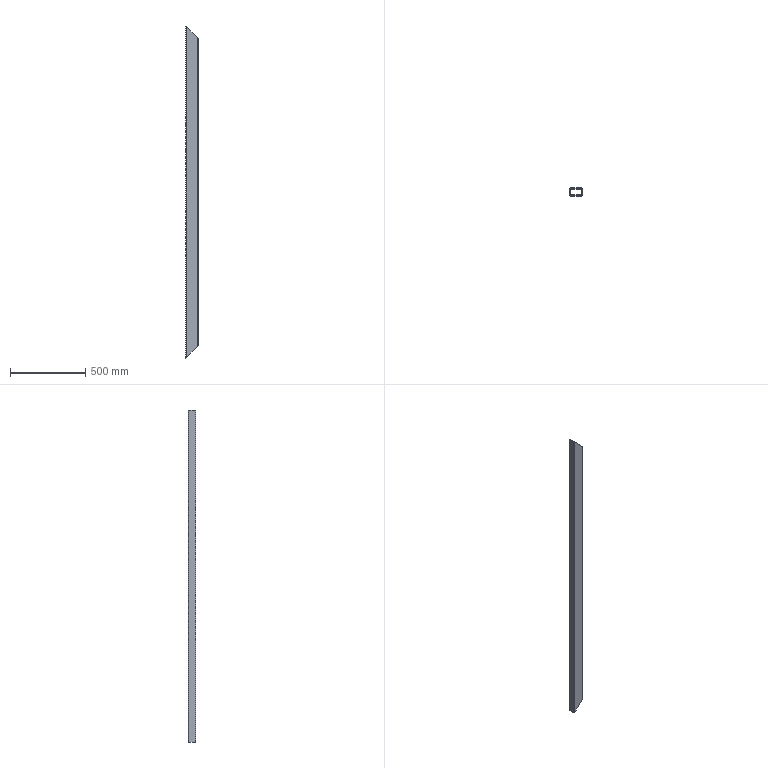Part | SolidWorks | features Extrusion 1, ICE 1, Shell 1 | 1 solid | 18 faces | box 80 x 50 x 2200 mm | volume 2025444 mm3 | plane 10 | cylinder 8 | commonest cylinder face diameters 2 x4 10 x4
STEP:
#1=CARTESIAN_POINT('',(-35.,21.,2195.));
#2=VERTEX_POINT('',#1);
#3=CARTESIAN_POINT('',(35.,21.,2125.));
#4=VERTEX_POINT('',#3);
#5=CARTESIAN_POINT('',(-2.5,21.,2162.5));
#6=DIRECTION('',(0.7071,0.,-0.7071));
#7=VECTOR('',#6,1000.);
#8=LINE('',#5,#7);
#9=EDGE_CURVE('',#2,#4,#8,.T.);
#10=ORIENTED_EDGE('',*,*,#9,.F.);
#11=CARTESIAN_POINT('',(-35.,21.,5.));
#12=VERTEX_POINT('',#11);
#13=CARTESIAN_POINT('',(-35.,21.,2200.));
#14=DIRECTION('',(0.,0.,-1.));
#15=VECTOR('',#14,1000.);
#16=LINE('',#13,#15);
#17=EDGE_CURVE('',#2,#12,#16,.T.);
#18=ORIENTED_EDGE('',*,*,#17,.T.);
#19=CARTESIAN_POINT('',(35.,21.,75.));
#20=VERTEX_POINT('',#19);
#21=CARTESIAN_POINT('',(1097.5,21.,1137.5));
#22=DIRECTION('',(-0.7071,0.,-0.7071));
#23=VECTOR('',#22,1000.);
#24=LINE('',#21,#23);
#25=EDGE_CURVE('',#20,#12,#24,.T.);
#26=ORIENTED_EDGE('',*,*,#25,.F.);
#27=CARTESIAN_POINT('',(35.,21.,2200.));
#28=DIRECTION('',(0.,0.,-1.));
#29=VECTOR('',#28,1000.);
#30=LINE('',#27,#29);
#31=EDGE_CURVE('',#4,#20,#30,.T.);
#32=ORIENTED_EDGE('',*,*,#31,.F.);
#33=EDGE_LOOP('',(#10,#18,#26,#32));
#34=FACE_OUTER_BOUND('',#33,.T.);
#35=CARTESIAN_POINT('',(35.,21.,2200.));
#36=DIRECTION('',(0.,-1.,0.));
#37=DIRECTION('',(1.,0.,0.));
#38=AXIS2_PLACEMENT_3D('',#35,#36,#37);
#39=PLANE('',#38);
#40=ADVANCED_FACE('',(#34),#39,.T.);
#41=CARTESIAN_POINT('',(36.,20.,2124.));
#42=VERTEX_POINT('',#41);
#43=CARTESIAN_POINT('',(36.,20.,76.));
#44=VERTEX_POINT('',#43);
#45=CARTESIAN_POINT('',(36.,20.,2200.));
#46=DIRECTION('',(0.,0.,-1.));
#47=VECTOR('',#46,1000.);
#48=LINE('',#45,#47);
#49=EDGE_CURVE('',#42,#44,#48,.T.);
#50=ORIENTED_EDGE('',*,*,#49,.F.);
#51=CARTESIAN_POINT('',(36.,20.,2124.));
#52=CARTESIAN_POINT('',(36.,20.586,2124.));
#53=CARTESIAN_POINT('',(35.586,21.,2124.414));
#54=CARTESIAN_POINT('',(35.,21.,2125.));
#55=(BOUNDED_CURVE()B_SPLINE_CURVE(3,(#51,#52,#53,#54),.UNSPECIFIED.,.F.,.T.)B_SPLINE_CURVE_WITH_KNOTS((4,4),(0.,1.571),.UNSPECIFIED.)CURVE()GEOMETRIC_REPRESENTATION_ITEM()RATIONAL_B_SPLINE_CURVE((1.,0.8047,0.8047,1.))REPRESENTATION_ITEM(''));
#56=EDGE_CURVE('',#42,#4,#55,.T.);
#57=ORIENTED_EDGE('',*,*,#56,.T.);
#58=ORIENTED_EDGE('',*,*,#31,.T.);
#59=CARTESIAN_POINT('',(35.,21.,75.));
#60=CARTESIAN_POINT('',(35.586,21.,75.586));
#61=CARTESIAN_POINT('',(36.,20.586,76.));
#62=CARTESIAN_POINT('',(36.,20.,76.));
#63=(BOUNDED_CURVE()B_SPLINE_CURVE(3,(#59,#60,#61,#62),.UNSPECIFIED.,.F.,.F.)B_SPLINE_CURVE_WITH_KNOTS((4,4),(1.571,3.142),.UNSPECIFIED.)CURVE()GEOMETRIC_REPRESENTATION_ITEM()RATIONAL_B_SPLINE_CURVE((1.,0.8047,0.8047,1.))REPRESENTATION_ITEM(''));
#64=EDGE_CURVE('',#20,#44,#63,.T.);
#65=ORIENTED_EDGE('',*,*,#64,.T.);
#66=EDGE_LOOP('',(#50,#57,#58,#65));
#67=FACE_OUTER_BOUND('',#66,.T.);
#68=CARTESIAN_POINT('',(35.,20.,2200.));
#69=DIRECTION('',(0.,0.,-1.));
#70=DIRECTION('',(-1.,0.,0.));
#71=AXIS2_PLACEMENT_3D('',#68,#69,#70);
#72=CYLINDRICAL_SURFACE('',#71,1.);
#73=ADVANCED_FACE('',(#67),#72,.F.);
#74=CARTESIAN_POINT('',(36.,-20.,2124.));
#75=VERTEX_POINT('',#74);
#76=CARTESIAN_POINT('',(36.,-20.,76.));
#77=VERTEX_POINT('',#76);
#78=CARTESIAN_POINT('',(36.,-20.,2200.));
#79=DIRECTION('',(0.,0.,-1.));
#80=VECTOR('',#79,1000.);
#81=LINE('',#78,#80);
#82=EDGE_CURVE('',#75,#77,#81,.T.);
#83=ORIENTED_EDGE('',*,*,#82,.F.);
#84=CARTESIAN_POINT('',(36.,20.,2124.));
#85=DIRECTION('',(0.,1.,0.));
#86=VECTOR('',#85,1000.);
#87=LINE('',#84,#86);
#88=EDGE_CURVE('',#75,#42,#87,.T.);
#89=ORIENTED_EDGE('',*,*,#88,.T.);
#90=ORIENTED_EDGE('',*,*,#49,.T.);
#91=CARTESIAN_POINT('',(36.,20.,76.));
#92=DIRECTION('',(0.,-1.,0.));
#93=VECTOR('',#92,1000.);
#94=LINE('',#91,#93);
#95=EDGE_CURVE('',#44,#77,#94,.T.);
#96=ORIENTED_EDGE('',*,*,#95,.T.);
#97=EDGE_LOOP('',(#83,#89,#90,#96));
#98=FACE_OUTER_BOUND('',#97,.T.);
#99=CARTESIAN_POINT('',(36.,20.,2200.));
#100=DIRECTION('',(1.,0.,0.));
#101=DIRECTION('',(0.,1.,0.));
#102=AXIS2_PLACEMENT_3D('',#99,#100,#101);
#103=PLANE('',#102);
#104=ADVANCED_FACE('',(#98),#103,.F.);
#105=CARTESIAN_POINT('',(35.,-21.,2125.));
#106=VERTEX_POINT('',#105);
#107=CARTESIAN_POINT('',(35.,-21.,75.));
#108=VERTEX_POINT('',#107);
#109=CARTESIAN_POINT('',(35.,-21.,2200.));
#110=DIRECTION('',(0.,0.,-1.));
#111=VECTOR('',#110,1000.);
#112=LINE('',#109,#111);
#113=EDGE_CURVE('',#106,#108,#112,.T.);
#114=ORIENTED_EDGE('',*,*,#113,.F.);
#115=CARTESIAN_POINT('',(35.,-21.,2125.));
#116=CARTESIAN_POINT('',(35.586,-21.,2124.414));
#117=CARTESIAN_POINT('',(36.,-20.586,2124.));
#118=CARTESIAN_POINT('',(36.,-20.,2124.));
#119=(BOUNDED_CURVE()B_SPLINE_CURVE(3,(#115,#116,#117,#118),.UNSPECIFIED.,.F.,.T.)B_SPLINE_CURVE_WITH_KNOTS((4,4),(4.712,6.283),.UNSPECIFIED.)CURVE()GEOMETRIC_REPRESENTATION_ITEM()RATIONAL_B_SPLINE_CURVE((1.,0.8047,0.8047,1.))REPRESENTATION_ITEM(''));
#120=EDGE_CURVE('',#106,#75,#119,.T.);
#121=ORIENTED_EDGE('',*,*,#120,.T.);
#122=ORIENTED_EDGE('',*,*,#82,.T.);
#123=CARTESIAN_POINT('',(36.,-20.,76.));
#124=CARTESIAN_POINT('',(36.,-20.586,76.));
#125=CARTESIAN_POINT('',(35.586,-21.,75.586));
#126=CARTESIAN_POINT('',(35.,-21.,75.));
#127=(BOUNDED_CURVE()B_SPLINE_CURVE(3,(#123,#124,#125,#126),.UNSPECIFIED.,.F.,.T.)B_SPLINE_CURVE_WITH_KNOTS((4,4),(3.142,4.712),.UNSPECIFIED.)CURVE()GEOMETRIC_REPRESENTATION_ITEM()RATIONAL_B_SPLINE_CURVE((1.,0.8047,0.8047,1.))REPRESENTATION_ITEM(''));
#128=EDGE_CURVE('',#77,#108,#127,.T.);
#129=ORIENTED_EDGE('',*,*,#128,.T.);
#130=EDGE_LOOP('',(#114,#121,#122,#129));
#131=FACE_OUTER_BOUND('',#130,.T.);
#132=CARTESIAN_POINT('',(35.,-20.,2200.));
#133=DIRECTION('',(0.,0.,-1.));
#134=DIRECTION('',(-1.,0.,0.));
#135=AXIS2_PLACEMENT_3D('',#132,#133,#134);
#136=CYLINDRICAL_SURFACE('',#135,1.);
#137=ADVANCED_FACE('',(#131),#136,.F.);
#138=CARTESIAN_POINT('',(-35.,-21.,2195.));
#139=VERTEX_POINT('',#138);
#140=CARTESIAN_POINT('',(-35.,-21.,5.));
#141=VERTEX_POINT('',#140);
#142=CARTESIAN_POINT('',(-35.,-21.,2200.));
#143=DIRECTION('',(0.,0.,-1.));
#144=VECTOR('',#143,1000.);
#145=LINE('',#142,#144);
#146=EDGE_CURVE('',#139,#141,#145,.T.);
#147=ORIENTED_EDGE('',*,*,#146,.F.);
#148=CARTESIAN_POINT('',(-2.5,-21.,2162.5));
#149=DIRECTION('',(0.7071,0.,-0.7071));
#150=VECTOR('',#149,1000.);
#151=LINE('',#148,#150);
#152=EDGE_CURVE('',#139,#106,#151,.T.);
#153=ORIENTED_EDGE('',*,*,#152,.T.);
#154=ORIENTED_EDGE('',*,*,#113,.T.);
#155=CARTESIAN_POINT('',(1097.5,-21.,1137.5));
#156=DIRECTION('',(-0.7071,0.,-0.7071));
#157=VECTOR('',#156,1000.);
#158=LINE('',#155,#157);
#159=EDGE_CURVE('',#108,#141,#158,.T.);
#160=ORIENTED_EDGE('',*,*,#159,.T.);
#161=EDGE_LOOP('',(#147,#153,#154,#160));
#162=FACE_OUTER_BOUND('',#161,.T.);
#163=CARTESIAN_POINT('',(35.,-21.,2200.));
#164=DIRECTION('',(0.,-1.,0.));
#165=DIRECTION('',(1.,0.,0.));
#166=AXIS2_PLACEMENT_3D('',#163,#164,#165);
#167=PLANE('',#166);
#168=ADVANCED_FACE('',(#162),#167,.F.);
#169=CARTESIAN_POINT('',(-36.,-20.,2196.));
#170=VERTEX_POINT('',#169);
#171=CARTESIAN_POINT('',(-36.,-20.,4.));
#172=VERTEX_POINT('',#171);
#173=CARTESIAN_POINT('',(-36.,-20.,2200.));
#174=DIRECTION('',(0.,0.,-1.));
#175=VECTOR('',#174,1000.);
#176=LINE('',#173,#175);
#177=EDGE_CURVE('',#170,#172,#176,.T.);
#178=ORIENTED_EDGE('',*,*,#177,.F.);
#179=CARTESIAN_POINT('',(-36.,-20.,2196.));
#180=CARTESIAN_POINT('',(-36.,-20.586,2196.));
#181=CARTESIAN_POINT('',(-35.586,-21.,2195.586));
#182=CARTESIAN_POINT('',(-35.,-21.,2195.));
#183=(BOUNDED_CURVE()B_SPLINE_CURVE(3,(#179,#180,#181,#182),.UNSPECIFIED.,.F.,.T.)B_SPLINE_CURVE_WITH_KNOTS((4,4),(3.142,4.712),.UNSPECIFIED.)CURVE()GEOMETRIC_REPRESENTATION_ITEM()RATIONAL_B_SPLINE_CURVE((1.,0.8047,0.8047,1.))REPRESENTATION_ITEM(''));
#184=EDGE_CURVE('',#170,#139,#183,.T.);
#185=ORIENTED_EDGE('',*,*,#184,.T.);
#186=ORIENTED_EDGE('',*,*,#146,.T.);
#187=CARTESIAN_POINT('',(-35.,-21.,5.));
#188=CARTESIAN_POINT('',(-35.586,-21.,4.414));
#189=CARTESIAN_POINT('',(-36.,-20.586,4.));
#190=CARTESIAN_POINT('',(-36.,-20.,4.));
#191=(BOUNDED_CURVE()B_SPLINE_CURVE(3,(#187,#188,#189,#190),.UNSPECIFIED.,.F.,.T.)B_SPLINE_CURVE_WITH_KNOTS((4,4),(4.712,6.283),.UNSPECIFIED.)CURVE()GEOMETRIC_REPRESENTATION_ITEM()RATIONAL_B_SPLINE_CURVE((1.,0.8047,0.8047,1.))REPRESENTATION_ITEM(''));
#192=EDGE_CURVE('',#141,#172,#191,.T.);
#193=ORIENTED_EDGE('',*,*,#192,.T.);
#194=EDGE_LOOP('',(#178,#185,#186,#193));
#195=FACE_OUTER_BOUND('',#194,.T.);
#196=CARTESIAN_POINT('',(-35.,-20.,2200.));
#197=DIRECTION('',(0.,0.,-1.));
#198=DIRECTION('',(-1.,0.,0.));
#199=AXIS2_PLACEMENT_3D('',#196,#197,#198);
#200=CYLINDRICAL_SURFACE('',#199,1.);
#201=ADVANCED_FACE('',(#195),#200,.F.);
#202=CARTESIAN_POINT('',(-36.,20.,2196.));
#203=VERTEX_POINT('',#202);
#204=CARTESIAN_POINT('',(-36.,20.,2196.));
#205=DIRECTION('',(0.,1.,0.));
#206=VECTOR('',#205,1000.);
#207=LINE('',#204,#206);
#208=EDGE_CURVE('',#170,#203,#207,.T.);
#209=ORIENTED_EDGE('',*,*,#208,.F.);
#210=ORIENTED_EDGE('',*,*,#177,.T.);
#211=CARTESIAN_POINT('',(-36.,20.,4.));
#212=VERTEX_POINT('',#211);
#213=CARTESIAN_POINT('',(-36.,20.,4.));
#214=DIRECTION('',(0.,-1.,0.));
#215=VECTOR('',#214,1000.);
#216=LINE('',#213,#215);
#217=EDGE_CURVE('',#212,#172,#216,.T.);
#218=ORIENTED_EDGE('',*,*,#217,.F.);
#219=CARTESIAN_POINT('',(-36.,20.,2200.));
#220=DIRECTION('',(0.,0.,-1.));
#221=VECTOR('',#220,1000.);
#222=LINE('',#219,#221);
#223=EDGE_CURVE('',#203,#212,#222,.T.);
#224=ORIENTED_EDGE('',*,*,#223,.F.);
#225=EDGE_LOOP('',(#209,#210,#218,#224));
#226=FACE_OUTER_BOUND('',#225,.T.);
#227=CARTESIAN_POINT('',(-36.,20.,2200.));
#228=DIRECTION('',(1.,0.,0.));
#229=DIRECTION('',(0.,1.,0.));
#230=AXIS2_PLACEMENT_3D('',#227,#228,#229);
#231=PLANE('',#230);
#232=ADVANCED_FACE('',(#226),#231,.T.);
#233=CARTESIAN_POINT('',(-36.,20.,2196.));
#234=CARTESIAN_POINT('',(-36.,20.586,2196.));
#235=CARTESIAN_POINT('',(-35.586,21.,2195.586));
#236=CARTESIAN_POINT('',(-35.,21.,2195.));
#237=(BOUNDED_CURVE()B_SPLINE_CURVE(3,(#233,#234,#235,#236),.UNSPECIFIED.,.F.,.T.)B_SPLINE_CURVE_WITH_KNOTS((4,4),(3.142,4.712),.UNSPECIFIED.)CURVE()GEOMETRIC_REPRESENTATION_ITEM()RATIONAL_B_SPLINE_CURVE((1.,0.8047,0.8047,1.))REPRESENTATION_ITEM(''));
#238=EDGE_CURVE('',#203,#2,#237,.T.);
#239=ORIENTED_EDGE('',*,*,#238,.F.);
#240=ORIENTED_EDGE('',*,*,#223,.T.);
#241=CARTESIAN_POINT('',(-35.,21.,5.));
#242=CARTESIAN_POINT('',(-35.586,21.,4.414));
#243=CARTESIAN_POINT('',(-36.,20.586,4.));
#244=CARTESIAN_POINT('',(-36.,20.,4.));
#245=(BOUNDED_CURVE()B_SPLINE_CURVE(3,(#241,#242,#243,#244),.UNSPECIFIED.,.F.,.T.)B_SPLINE_CURVE_WITH_KNOTS((4,4),(4.712,6.283),.UNSPECIFIED.)CURVE()GEOMETRIC_REPRESENTATION_ITEM()RATIONAL_B_SPLINE_CURVE((1.,0.8047,0.8047,1.))REPRESENTATION_ITEM(''));
#246=EDGE_CURVE('',#12,#212,#245,.T.);
#247=ORIENTED_EDGE('',*,*,#246,.F.);
#248=ORIENTED_EDGE('',*,*,#17,.F.);
#249=EDGE_LOOP('',(#239,#240,#247,#248));
#250=FACE_OUTER_BOUND('',#249,.T.);
#251=CARTESIAN_POINT('',(-35.,20.,2200.));
#252=DIRECTION('',(0.,0.,-1.));
#253=DIRECTION('',(-1.,0.,0.));
#254=AXIS2_PLACEMENT_3D('',#251,#252,#253);
#255=CYLINDRICAL_SURFACE('',#254,1.);
#256=ADVANCED_FACE('',(#250),#255,.F.);
#257=CARTESIAN_POINT('',(-35.,-25.,5.));
#258=VERTEX_POINT('',#257);
#259=CARTESIAN_POINT('',(-40.,-20.,0.));
#260=VERTEX_POINT('',#259);
#261=CARTESIAN_POINT('',(-35.,-25.,5.));
#262=CARTESIAN_POINT('',(-37.929,-25.,2.071));
#263=CARTESIAN_POINT('',(-40.,-22.929,0.));
#264=CARTESIAN_POINT('',(-40.,-20.,0.));
#265=(BOUNDED_CURVE()B_SPLINE_CURVE(3,(#261,#262,#263,#264),.UNSPECIFIED.,.F.,.T.)B_SPLINE_CURVE_WITH_KNOTS((4,4),(4.712,6.283),.UNSPECIFIED.)CURVE()GEOMETRIC_REPRESENTATION_ITEM()RATIONAL_B_SPLINE_CURVE((1.,0.8047,0.8047,1.))REPRESENTATION_ITEM(''));
#266=EDGE_CURVE('',#258,#260,#265,.T.);
#267=ORIENTED_EDGE('',*,*,#266,.T.);
#268=CARTESIAN_POINT('',(-40.,20.,0.));
#269=VERTEX_POINT('',#268);
#270=CARTESIAN_POINT('',(-40.,20.,0.));
#271=DIRECTION('',(0.,-1.,0.));
#272=VECTOR('',#271,1000.);
#273=LINE('',#270,#272);
#274=EDGE_CURVE('',#269,#260,#273,.T.);
#275=ORIENTED_EDGE('',*,*,#274,.F.);
#276=CARTESIAN_POINT('',(-35.,25.,5.));
#277=VERTEX_POINT('',#276);
#278=CARTESIAN_POINT('',(-35.,25.,5.));
#279=CARTESIAN_POINT('',(-37.929,25.,2.071));
#280=CARTESIAN_POINT('',(-40.,22.929,0.));
#281=CARTESIAN_POINT('',(-40.,20.,0.));
#282=(BOUNDED_CURVE()B_SPLINE_CURVE(3,(#278,#279,#280,#281),.UNSPECIFIED.,.F.,.T.)B_SPLINE_CURVE_WITH_KNOTS((4,4),(4.712,6.283),.UNSPECIFIED.)CURVE()GEOMETRIC_REPRESENTATION_ITEM()RATIONAL_B_SPLINE_CURVE((1.,0.8047,0.8047,1.))REPRESENTATION_ITEM(''));
#283=EDGE_CURVE('',#277,#269,#282,.T.);
#284=ORIENTED_EDGE('',*,*,#283,.F.);
#285=CARTESIAN_POINT('',(35.,25.,75.));
#286=VERTEX_POINT('',#285);
#287=CARTESIAN_POINT('',(1097.5,25.,1137.5));
#288=DIRECTION('',(-0.7071,0.,-0.7071));
#289=VECTOR('',#288,1000.);
#290=LINE('',#287,#289);
#291=EDGE_CURVE('',#286,#277,#290,.T.);
#292=ORIENTED_EDGE('',*,*,#291,.F.);
#293=CARTESIAN_POINT('',(40.,20.,80.));
#294=VERTEX_POINT('',#293);
#295=CARTESIAN_POINT('',(35.,25.,75.));
#296=CARTESIAN_POINT('',(37.929,25.,77.929));
#297=CARTESIAN_POINT('',(40.,22.929,80.));
#298=CARTESIAN_POINT('',(40.,20.,80.));
#299=(BOUNDED_CURVE()B_SPLINE_CURVE(3,(#295,#296,#297,#298),.UNSPECIFIED.,.F.,.T.)B_SPLINE_CURVE_WITH_KNOTS((4,4),(1.571,3.142),.UNSPECIFIED.)CURVE()GEOMETRIC_REPRESENTATION_ITEM()RATIONAL_B_SPLINE_CURVE((1.,0.8047,0.8047,1.))REPRESENTATION_ITEM(''));
#300=EDGE_CURVE('',#286,#294,#299,.T.);
#301=ORIENTED_EDGE('',*,*,#300,.T.);
#302=CARTESIAN_POINT('',(40.,-20.,80.));
#303=VERTEX_POINT('',#302);
#304=CARTESIAN_POINT('',(40.,1975.,80.));
#305=DIRECTION('',(0.,-1.,0.));
#306=VECTOR('',#305,1000.);
#307=LINE('',#304,#306);
#308=EDGE_CURVE('',#294,#303,#307,.T.);
#309=ORIENTED_EDGE('',*,*,#308,.T.);
#310=CARTESIAN_POINT('',(35.,-25.,75.));
#311=VERTEX_POINT('',#310);
#312=CARTESIAN_POINT('',(40.,-20.,80.));
#313=CARTESIAN_POINT('',(40.,-22.929,80.));
#314=CARTESIAN_POINT('',(37.929,-25.,77.929));
#315=CARTESIAN_POINT('',(35.,-25.,75.));
#316=(BOUNDED_CURVE()B_SPLINE_CURVE(3,(#312,#313,#314,#315),.UNSPECIFIED.,.F.,.T.)B_SPLINE_CURVE_WITH_KNOTS((4,4),(3.142,4.712),.UNSPECIFIED.)CURVE()GEOMETRIC_REPRESENTATION_ITEM()RATIONAL_B_SPLINE_CURVE((1.,0.8047,0.8047,1.))REPRESENTATION_ITEM(''));
#317=EDGE_CURVE('',#303,#311,#316,.T.);
#318=ORIENTED_EDGE('',*,*,#317,.T.);
#319=CARTESIAN_POINT('',(-40.,-25.,0.));
#320=DIRECTION('',(-0.7071,0.,-0.7071));
#321=VECTOR('',#320,1000.);
#322=LINE('',#319,#321);
#323=EDGE_CURVE('',#311,#258,#322,.T.);
#324=ORIENTED_EDGE('',*,*,#323,.T.);
#325=EDGE_LOOP('',(#267,#275,#284,#292,#301,#309,#318,#324));
#326=FACE_OUTER_BOUND('',#325,.T.);
#327=ORIENTED_EDGE('',*,*,#246,.T.);
#328=ORIENTED_EDGE('',*,*,#217,.T.);
#329=ORIENTED_EDGE('',*,*,#192,.F.);
#330=ORIENTED_EDGE('',*,*,#159,.F.);
#331=ORIENTED_EDGE('',*,*,#128,.F.);
#332=ORIENTED_EDGE('',*,*,#95,.F.);
#333=ORIENTED_EDGE('',*,*,#64,.F.);
#334=ORIENTED_EDGE('',*,*,#25,.T.);
#335=EDGE_LOOP('',(#327,#328,#329,#330,#331,#332,#333,#334));
#336=FACE_BOUND('',#335,.T.);
#337=CARTESIAN_POINT('',(-40.,1975.,0.));
#338=DIRECTION('',(-0.7071,0.,0.7071));
#339=DIRECTION('',(0.7071,0.,0.7071));
#340=AXIS2_PLACEMENT_3D('',#337,#338,#339);
#341=PLANE('',#340);
#342=ADVANCED_FACE('',(#326,#336),#341,.F.);
#343=CARTESIAN_POINT('',(-40.,-20.,2200.));
#344=VERTEX_POINT('',#343);
#345=CARTESIAN_POINT('',(-35.,-25.,2195.));
#346=VERTEX_POINT('',#345);
#347=CARTESIAN_POINT('',(-40.,-20.,2200.));
#348=CARTESIAN_POINT('',(-40.,-22.929,2200.));
#349=CARTESIAN_POINT('',(-37.929,-25.,2197.929));
#350=CARTESIAN_POINT('',(-35.,-25.,2195.));
#351=(BOUNDED_CURVE()B_SPLINE_CURVE(3,(#347,#348,#349,#350),.UNSPECIFIED.,.F.,.F.)B_SPLINE_CURVE_WITH_KNOTS((4,4),(3.142,4.712),.UNSPECIFIED.)CURVE()GEOMETRIC_REPRESENTATION_ITEM()RATIONAL_B_SPLINE_CURVE((1.,0.8047,0.8047,1.))REPRESENTATION_ITEM(''));
#352=EDGE_CURVE('',#344,#346,#351,.T.);
#353=ORIENTED_EDGE('',*,*,#352,.T.);
#354=CARTESIAN_POINT('',(35.,-25.,2125.));
#355=VERTEX_POINT('',#354);
#356=CARTESIAN_POINT('',(-40.,-25.,2200.));
#357=DIRECTION('',(0.7071,0.,-0.7071));
#358=VECTOR('',#357,1000.);
#359=LINE('',#356,#358);
#360=EDGE_CURVE('',#346,#355,#359,.T.);
#361=ORIENTED_EDGE('',*,*,#360,.T.);
#362=CARTESIAN_POINT('',(40.,-20.,2120.));
#363=VERTEX_POINT('',#362);
#364=CARTESIAN_POINT('',(35.,-25.,2125.));
#365=CARTESIAN_POINT('',(37.929,-25.,2122.071));
#366=CARTESIAN_POINT('',(40.,-22.929,2120.));
#367=CARTESIAN_POINT('',(40.,-20.,2120.));
#368=(BOUNDED_CURVE()B_SPLINE_CURVE(3,(#364,#365,#366,#367),.UNSPECIFIED.,.F.,.T.)B_SPLINE_CURVE_WITH_KNOTS((4,4),(4.712,6.283),.UNSPECIFIED.)CURVE()GEOMETRIC_REPRESENTATION_ITEM()RATIONAL_B_SPLINE_CURVE((1.,0.8047,0.8047,1.))REPRESENTATION_ITEM(''));
#369=EDGE_CURVE('',#355,#363,#368,.T.);
#370=ORIENTED_EDGE('',*,*,#369,.T.);
#371=CARTESIAN_POINT('',(40.,20.,2120.));
#372=VERTEX_POINT('',#371);
#373=CARTESIAN_POINT('',(40.,1975.,2120.));
#374=DIRECTION('',(0.,-1.,0.));
#375=VECTOR('',#374,1000.);
#376=LINE('',#373,#375);
#377=EDGE_CURVE('',#372,#363,#376,.T.);
#378=ORIENTED_EDGE('',*,*,#377,.F.);
#379=CARTESIAN_POINT('',(35.,25.,2125.));
#380=VERTEX_POINT('',#379);
#381=CARTESIAN_POINT('',(40.,20.,2120.));
#382=CARTESIAN_POINT('',(40.,22.929,2120.));
#383=CARTESIAN_POINT('',(37.929,25.,2122.071));
#384=CARTESIAN_POINT('',(35.,25.,2125.));
#385=(BOUNDED_CURVE()B_SPLINE_CURVE(3,(#381,#382,#383,#384),.UNSPECIFIED.,.F.,.T.)B_SPLINE_CURVE_WITH_KNOTS((4,4),(0.,1.571),.UNSPECIFIED.)CURVE()GEOMETRIC_REPRESENTATION_ITEM()RATIONAL_B_SPLINE_CURVE((1.,0.8047,0.8047,1.))REPRESENTATION_ITEM(''));
#386=EDGE_CURVE('',#372,#380,#385,.T.);
#387=ORIENTED_EDGE('',*,*,#386,.T.);
#388=CARTESIAN_POINT('',(-35.,25.,2195.));
#389=VERTEX_POINT('',#388);
#390=CARTESIAN_POINT('',(-2.5,25.,2162.5));
#391=DIRECTION('',(0.7071,0.,-0.7071));
#392=VECTOR('',#391,1000.);
#393=LINE('',#390,#392);
#394=EDGE_CURVE('',#389,#380,#393,.T.);
#395=ORIENTED_EDGE('',*,*,#394,.F.);
#396=CARTESIAN_POINT('',(-40.,20.,2200.));
#397=VERTEX_POINT('',#396);
#398=CARTESIAN_POINT('',(-40.,20.,2200.));
#399=CARTESIAN_POINT('',(-40.,22.929,2200.));
#400=CARTESIAN_POINT('',(-37.929,25.,2197.929));
#401=CARTESIAN_POINT('',(-35.,25.,2195.));
#402=(BOUNDED_CURVE()B_SPLINE_CURVE(3,(#398,#399,#400,#401),.UNSPECIFIED.,.F.,.F.)B_SPLINE_CURVE_WITH_KNOTS((4,4),(3.142,4.712),.UNSPECIFIED.)CURVE()GEOMETRIC_REPRESENTATION_ITEM()RATIONAL_B_SPLINE_CURVE((1.,0.8047,0.8047,1.))REPRESENTATION_ITEM(''));
#403=EDGE_CURVE('',#397,#389,#402,.T.);
#404=ORIENTED_EDGE('',*,*,#403,.F.);
#405=CARTESIAN_POINT('',(-40.,20.,2200.));
#406=DIRECTION('',(0.,-1.,0.));
#407=VECTOR('',#406,1000.);
#408=LINE('',#405,#407);
#409=EDGE_CURVE('',#397,#344,#408,.T.);
#410=ORIENTED_EDGE('',*,*,#409,.T.);
#411=EDGE_LOOP('',(#353,#361,#370,#378,#387,#395,#404,#410));
#412=FACE_OUTER_BOUND('',#411,.T.);
#413=ORIENTED_EDGE('',*,*,#238,.T.);
#414=ORIENTED_EDGE('',*,*,#9,.T.);
#415=ORIENTED_EDGE('',*,*,#56,.F.);
#416=ORIENTED_EDGE('',*,*,#88,.F.);
#417=ORIENTED_EDGE('',*,*,#120,.F.);
#418=ORIENTED_EDGE('',*,*,#152,.F.);
#419=ORIENTED_EDGE('',*,*,#184,.F.);
#420=ORIENTED_EDGE('',*,*,#208,.T.);
#421=EDGE_LOOP('',(#413,#414,#415,#416,#417,#418,#419,#420));
#422=FACE_BOUND('',#421,.T.);
#423=CARTESIAN_POINT('',(-40.,1975.,2200.));
#424=DIRECTION('',(-0.7071,0.,-0.7071));
#425=DIRECTION('',(-0.7071,0.,0.7071));
#426=AXIS2_PLACEMENT_3D('',#423,#424,#425);
#427=PLANE('',#426);
#428=ADVANCED_FACE('',(#412,#422),#427,.F.);
#429=CARTESIAN_POINT('',(-40.,20.,2200.));
#430=DIRECTION('',(0.,0.,-1.));
#431=VECTOR('',#430,1000.);
#432=LINE('',#429,#431);
#433=EDGE_CURVE('',#397,#269,#432,.T.);
#434=ORIENTED_EDGE('',*,*,#433,.F.);
#435=ORIENTED_EDGE('',*,*,#403,.T.);
#436=CARTESIAN_POINT('',(-35.,25.,2200.));
#437=DIRECTION('',(0.,0.,-1.));
#438=VECTOR('',#437,1000.);
#439=LINE('',#436,#438);
#440=EDGE_CURVE('',#389,#277,#439,.T.);
#441=ORIENTED_EDGE('',*,*,#440,.T.);
#442=ORIENTED_EDGE('',*,*,#283,.T.);
#443=EDGE_LOOP('',(#434,#435,#441,#442));
#444=FACE_OUTER_BOUND('',#443,.T.);
#445=CARTESIAN_POINT('',(-35.,20.,2200.));
#446=DIRECTION('',(0.,0.,-1.));
#447=DIRECTION('',(-1.,0.,0.));
#448=AXIS2_PLACEMENT_3D('',#445,#446,#447);
#449=CYLINDRICAL_SURFACE('',#448,5.);
#450=ADVANCED_FACE('',(#444),#449,.T.);
#451=ORIENTED_EDGE('',*,*,#274,.T.);
#452=CARTESIAN_POINT('',(-40.,-20.,2200.));
#453=DIRECTION('',(0.,0.,-1.));
#454=VECTOR('',#453,1000.);
#455=LINE('',#452,#454);
#456=EDGE_CURVE('',#344,#260,#455,.T.);
#457=ORIENTED_EDGE('',*,*,#456,.F.);
#458=ORIENTED_EDGE('',*,*,#409,.F.);
#459=ORIENTED_EDGE('',*,*,#433,.T.);
#460=EDGE_LOOP('',(#451,#457,#458,#459));
#461=FACE_OUTER_BOUND('',#460,.T.);
#462=CARTESIAN_POINT('',(-40.,20.,2200.));
#463=DIRECTION('',(1.,0.,0.));
#464=DIRECTION('',(0.,1.,0.));
#465=AXIS2_PLACEMENT_3D('',#462,#463,#464);
#466=PLANE('',#465);
#467=ADVANCED_FACE('',(#461),#466,.F.);
#468=ORIENTED_EDGE('',*,*,#352,.F.);
#469=ORIENTED_EDGE('',*,*,#456,.T.);
#470=ORIENTED_EDGE('',*,*,#266,.F.);
#471=CARTESIAN_POINT('',(-35.,-25.,2200.));
#472=DIRECTION('',(0.,0.,-1.));
#473=VECTOR('',#472,1000.);
#474=LINE('',#471,#473);
#475=EDGE_CURVE('',#346,#258,#474,.T.);
#476=ORIENTED_EDGE('',*,*,#475,.F.);
#477=EDGE_LOOP('',(#468,#469,#470,#476));
#478=FACE_OUTER_BOUND('',#477,.T.);
#479=CARTESIAN_POINT('',(-35.,-20.,2200.));
#480=DIRECTION('',(0.,0.,-1.));
#481=DIRECTION('',(-1.,0.,0.));
#482=AXIS2_PLACEMENT_3D('',#479,#480,#481);
#483=CYLINDRICAL_SURFACE('',#482,5.);
#484=ADVANCED_FACE('',(#478),#483,.T.);
#485=ORIENTED_EDGE('',*,*,#360,.F.);
#486=ORIENTED_EDGE('',*,*,#475,.T.);
#487=ORIENTED_EDGE('',*,*,#323,.F.);
#488=CARTESIAN_POINT('',(35.,-25.,2200.));
#489=DIRECTION('',(0.,0.,-1.));
#490=VECTOR('',#489,1000.);
#491=LINE('',#488,#490);
#492=EDGE_CURVE('',#355,#311,#491,.T.);
#493=ORIENTED_EDGE('',*,*,#492,.F.);
#494=EDGE_LOOP('',(#485,#486,#487,#493));
#495=FACE_OUTER_BOUND('',#494,.T.);
#496=CARTESIAN_POINT('',(35.,-25.,2200.));
#497=DIRECTION('',(0.,-1.,0.));
#498=DIRECTION('',(1.,0.,0.));
#499=AXIS2_PLACEMENT_3D('',#496,#497,#498);
#500=PLANE('',#499);
#501=ADVANCED_FACE('',(#495),#500,.T.);
#502=ORIENTED_EDGE('',*,*,#369,.F.);
#503=ORIENTED_EDGE('',*,*,#492,.T.);
#504=ORIENTED_EDGE('',*,*,#317,.F.);
#505=CARTESIAN_POINT('',(40.,-20.,2200.));
#506=DIRECTION('',(0.,0.,-1.));
#507=VECTOR('',#506,1000.);
#508=LINE('',#505,#507);
#509=EDGE_CURVE('',#363,#303,#508,.T.);
#510=ORIENTED_EDGE('',*,*,#509,.F.);
#511=EDGE_LOOP('',(#502,#503,#504,#510));
#512=FACE_OUTER_BOUND('',#511,.T.);
#513=CARTESIAN_POINT('',(35.,-20.,2200.));
#514=DIRECTION('',(0.,0.,-1.));
#515=DIRECTION('',(-1.,0.,0.));
#516=AXIS2_PLACEMENT_3D('',#513,#514,#515);
#517=CYLINDRICAL_SURFACE('',#516,5.);
#518=ADVANCED_FACE('',(#512),#517,.T.);
#519=ORIENTED_EDGE('',*,*,#377,.T.);
#520=ORIENTED_EDGE('',*,*,#509,.T.);
#521=ORIENTED_EDGE('',*,*,#308,.F.);
#522=CARTESIAN_POINT('',(40.,20.,2200.));
#523=DIRECTION('',(0.,0.,-1.));
#524=VECTOR('',#523,1000.);
#525=LINE('',#522,#524);
#526=EDGE_CURVE('',#372,#294,#525,.T.);
#527=ORIENTED_EDGE('',*,*,#526,.F.);
#528=EDGE_LOOP('',(#519,#520,#521,#527));
#529=FACE_OUTER_BOUND('',#528,.T.);
#530=CARTESIAN_POINT('',(40.,20.,2200.));
#531=DIRECTION('',(1.,0.,0.));
#532=DIRECTION('',(0.,1.,0.));
#533=AXIS2_PLACEMENT_3D('',#530,#531,#532);
#534=PLANE('',#533);
#535=ADVANCED_FACE('',(#529),#534,.T.);
#536=ORIENTED_EDGE('',*,*,#386,.F.);
#537=ORIENTED_EDGE('',*,*,#526,.T.);
#538=ORIENTED_EDGE('',*,*,#300,.F.);
#539=CARTESIAN_POINT('',(35.,25.,2200.));
#540=DIRECTION('',(0.,0.,-1.));
#541=VECTOR('',#540,1000.);
#542=LINE('',#539,#541);
#543=EDGE_CURVE('',#380,#286,#542,.T.);
#544=ORIENTED_EDGE('',*,*,#543,.F.);
#545=EDGE_LOOP('',(#536,#537,#538,#544));
#546=FACE_OUTER_BOUND('',#545,.T.);
#547=CARTESIAN_POINT('',(35.,20.,2200.));
#548=DIRECTION('',(0.,0.,-1.));
#549=DIRECTION('',(-1.,0.,0.));
#550=AXIS2_PLACEMENT_3D('',#547,#548,#549);
#551=CYLINDRICAL_SURFACE('',#550,5.);
#552=ADVANCED_FACE('',(#546),#551,.T.);
#553=ORIENTED_EDGE('',*,*,#440,.F.);
#554=ORIENTED_EDGE('',*,*,#394,.T.);
#555=ORIENTED_EDGE('',*,*,#543,.T.);
#556=ORIENTED_EDGE('',*,*,#291,.T.);
#557=EDGE_LOOP('',(#553,#554,#555,#556));
#558=FACE_OUTER_BOUND('',#557,.T.);
#559=CARTESIAN_POINT('',(35.,25.,2200.));
#560=DIRECTION('',(0.,-1.,0.));
#561=DIRECTION('',(1.,0.,0.));
#562=AXIS2_PLACEMENT_3D('',#559,#560,#561);
#563=PLANE('',#562);
#564=ADVANCED_FACE('',(#558),#563,.F.);
#565=CLOSED_SHELL('',(#40,#73,#104,#137,#168,#201,#232,#256,#342,#428,#450,#467,#484,#501,#518,#535,#552,#564));
#566=MANIFOLD_SOLID_BREP('',#565);
#567=CARTESIAN_POINT('',(0.,0.,0.));
#568=DIRECTION('',(0.,0.,1.));
#569=DIRECTION('',(1.,0.,0.));
#570=AXIS2_PLACEMENT_3D('',#567,#568,#569);
#571=(LENGTH_UNIT()NAMED_UNIT(*)SI_UNIT(.MILLI.,.METRE.));
#572=UNCERTAINTY_MEASURE_WITH_UNIT(LENGTH_MEASURE(0.00001),#571,'','');
#573=(NAMED_UNIT(*)PLANE_ANGLE_UNIT()SI_UNIT($,.RADIAN.));
#574=(NAMED_UNIT(*)SI_UNIT($,.STERADIAN.)SOLID_ANGLE_UNIT());
#575=(GEOMETRIC_REPRESENTATION_CONTEXT(3)GLOBAL_UNCERTAINTY_ASSIGNED_CONTEXT((#572))GLOBAL_UNIT_ASSIGNED_CONTEXT((#571,#573,#574))REPRESENTATION_CONTEXT('',''));
#576=ADVANCED_BREP_SHAPE_REPRESENTATION('',(#566,#570),#575);